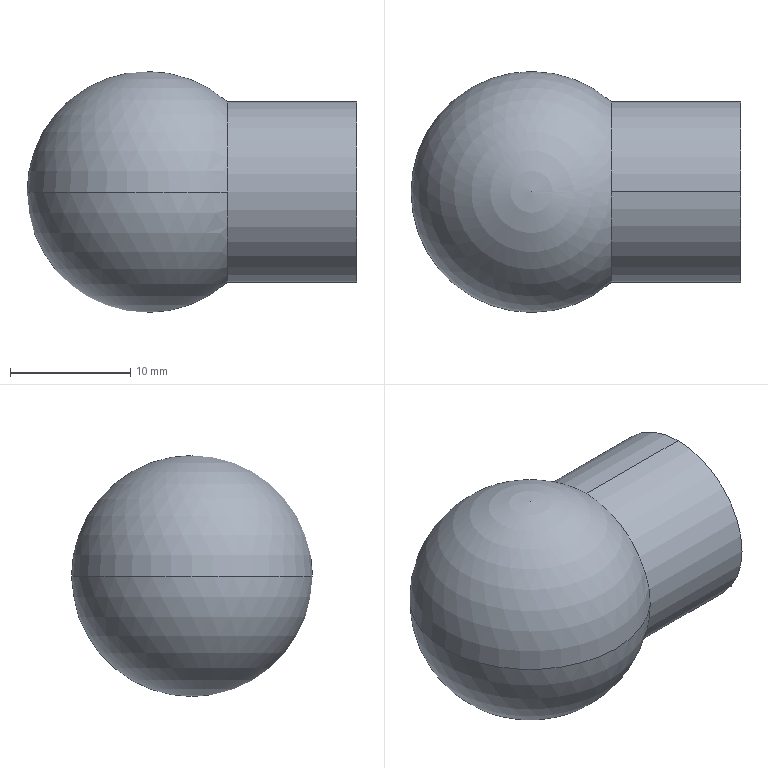Part | SolidWorks | features Revolution 2 | 1 solid | 6 faces | box 27.386 x 20 x 20 mm | volume 5453 mm3 | sphere 4 | cylinder 2 | commonest cylinder face diameters 15 x2
STEP:
#1=CARTESIAN_POINT('',(0.,-10.,0.));
#2=VERTEX_POINT('',#1);
#3=CARTESIAN_POINT('',(6.614,-7.5,0.));
#4=VERTEX_POINT('',#3);
#5=CARTESIAN_POINT('',(0.,0.,0.));
#6=DIRECTION('',(0.,0.,1.));
#7=DIRECTION('',(1.,0.,0.));
#8=AXIS2_PLACEMENT_3D('',#5,#6,#7);
#9=CIRCLE('',#8,10.);
#10=EDGE_CURVE('',#2,#4,#9,.T.);
#11=ORIENTED_EDGE('',*,*,#10,.F.);
#12=CARTESIAN_POINT('',(0.,10.,0.));
#13=VERTEX_POINT('',#12);
#14=CARTESIAN_POINT('',(0.,0.,0.));
#15=DIRECTION('',(0.,0.,-1.));
#16=DIRECTION('',(-1.,0.,0.));
#17=AXIS2_PLACEMENT_3D('',#14,#15,#16);
#18=CIRCLE('',#17,10.);
#19=EDGE_CURVE('',#2,#13,#18,.T.);
#20=ORIENTED_EDGE('',*,*,#19,.T.);
#21=CARTESIAN_POINT('',(6.614,7.5,0.));
#22=VERTEX_POINT('',#21);
#23=CARTESIAN_POINT('',(0.,0.,0.));
#24=DIRECTION('',(0.,0.,1.));
#25=DIRECTION('',(1.,0.,0.));
#26=AXIS2_PLACEMENT_3D('',#23,#24,#25);
#27=CIRCLE('',#26,10.);
#28=EDGE_CURVE('',#22,#13,#27,.T.);
#29=ORIENTED_EDGE('',*,*,#28,.F.);
#30=CARTESIAN_POINT('',(6.614,0.,-7.5));
#31=VERTEX_POINT('',#30);
#32=CARTESIAN_POINT('',(6.614,0.,0.));
#33=DIRECTION('',(1.,0.,0.));
#34=DIRECTION('',(0.,0.,-1.));
#35=AXIS2_PLACEMENT_3D('',#32,#33,#34);
#36=CIRCLE('',#35,7.5);
#37=EDGE_CURVE('',#31,#22,#36,.T.);
#38=ORIENTED_EDGE('',*,*,#37,.F.);
#39=CARTESIAN_POINT('',(6.614,0.,0.));
#40=DIRECTION('',(1.,0.,0.));
#41=DIRECTION('',(0.,0.,-1.));
#42=AXIS2_PLACEMENT_3D('',#39,#40,#41);
#43=CIRCLE('',#42,7.5);
#44=EDGE_CURVE('',#4,#31,#43,.T.);
#45=ORIENTED_EDGE('',*,*,#44,.F.);
#46=EDGE_LOOP('',(#11,#20,#29,#38,#45));
#47=FACE_OUTER_BOUND('',#46,.T.);
#48=CARTESIAN_POINT('',(0.,0.,0.));
#49=DIRECTION('',(0.,0.,-1.));
#50=DIRECTION('',(1.,0.,0.));
#51=AXIS2_PLACEMENT_3D('',#48,#49,#50);
#52=SPHERICAL_SURFACE('',#51,10.);
#53=ADVANCED_FACE('',(#47),#52,.T.);
#54=ORIENTED_EDGE('',*,*,#37,.T.);
#55=CARTESIAN_POINT('',(6.614,0.,7.5));
#56=VERTEX_POINT('',#55);
#57=CARTESIAN_POINT('',(6.614,0.,0.));
#58=DIRECTION('',(1.,0.,0.));
#59=DIRECTION('',(0.,0.,-1.));
#60=AXIS2_PLACEMENT_3D('',#57,#58,#59);
#61=CIRCLE('',#60,7.5);
#62=EDGE_CURVE('',#22,#56,#61,.T.);
#63=ORIENTED_EDGE('',*,*,#62,.T.);
#64=CARTESIAN_POINT('',(17.386,0.,7.5));
#65=VERTEX_POINT('',#64);
#66=CARTESIAN_POINT('',(27.638,0.,7.5));
#67=DIRECTION('',(1.,0.,0.));
#68=VECTOR('',#67,1000.);
#69=LINE('',#66,#68);
#70=EDGE_CURVE('',#56,#65,#69,.T.);
#71=ORIENTED_EDGE('',*,*,#70,.T.);
#72=CARTESIAN_POINT('',(17.386,7.5,0.));
#73=VERTEX_POINT('',#72);
#74=CARTESIAN_POINT('',(17.386,0.,0.));
#75=DIRECTION('',(1.,0.,0.));
#76=DIRECTION('',(0.,0.,-1.));
#77=AXIS2_PLACEMENT_3D('',#74,#75,#76);
#78=CIRCLE('',#77,7.5);
#79=EDGE_CURVE('',#73,#65,#78,.T.);
#80=ORIENTED_EDGE('',*,*,#79,.F.);
#81=CARTESIAN_POINT('',(17.386,0.,-7.5));
#82=VERTEX_POINT('',#81);
#83=CARTESIAN_POINT('',(17.386,0.,0.));
#84=DIRECTION('',(1.,0.,0.));
#85=DIRECTION('',(0.,0.,-1.));
#86=AXIS2_PLACEMENT_3D('',#83,#84,#85);
#87=CIRCLE('',#86,7.5);
#88=EDGE_CURVE('',#82,#73,#87,.T.);
#89=ORIENTED_EDGE('',*,*,#88,.F.);
#90=CARTESIAN_POINT('',(27.638,0.,-7.5));
#91=DIRECTION('',(1.,0.,0.));
#92=VECTOR('',#91,1000.);
#93=LINE('',#90,#92);
#94=EDGE_CURVE('',#31,#82,#93,.T.);
#95=ORIENTED_EDGE('',*,*,#94,.F.);
#96=EDGE_LOOP('',(#54,#63,#71,#80,#89,#95));
#97=FACE_OUTER_BOUND('',#96,.T.);
#98=CARTESIAN_POINT('',(27.638,0.,0.));
#99=DIRECTION('',(1.,0.,0.));
#100=DIRECTION('',(0.,0.,-1.));
#101=AXIS2_PLACEMENT_3D('',#98,#99,#100);
#102=CYLINDRICAL_SURFACE('',#101,7.5);
#103=ADVANCED_FACE('',(#97),#102,.T.);
#104=CARTESIAN_POINT('',(14.,0.,0.));
#105=VERTEX_POINT('',#104);
#106=CARTESIAN_POINT('',(17.386,-7.5,0.));
#107=VERTEX_POINT('',#106);
#108=CARTESIAN_POINT('',(24.,0.,0.));
#109=DIRECTION('',(0.,0.,1.));
#110=DIRECTION('',(1.,0.,0.));
#111=AXIS2_PLACEMENT_3D('',#108,#109,#110);
#112=CIRCLE('',#111,10.);
#113=EDGE_CURVE('',#105,#107,#112,.T.);
#114=ORIENTED_EDGE('',*,*,#113,.F.);
#115=CARTESIAN_POINT('',(24.,0.,0.));
#116=DIRECTION('',(0.,0.,-1.));
#117=DIRECTION('',(0.,1.,0.));
#118=AXIS2_PLACEMENT_3D('',#115,#116,#117);
#119=CIRCLE('',#118,10.);
#120=EDGE_CURVE('',#105,#73,#119,.T.);
#121=ORIENTED_EDGE('',*,*,#120,.T.);
#122=ORIENTED_EDGE('',*,*,#79,.T.);
#123=CARTESIAN_POINT('',(17.386,0.,0.));
#124=DIRECTION('',(1.,0.,0.));
#125=DIRECTION('',(0.,0.,-1.));
#126=AXIS2_PLACEMENT_3D('',#123,#124,#125);
#127=CIRCLE('',#126,7.5);
#128=EDGE_CURVE('',#65,#107,#127,.T.);
#129=ORIENTED_EDGE('',*,*,#128,.T.);
#130=EDGE_LOOP('',(#114,#121,#122,#129));
#131=FACE_OUTER_BOUND('',#130,.T.);
#132=CARTESIAN_POINT('',(24.,0.,0.));
#133=DIRECTION('',(0.,0.,-1.));
#134=DIRECTION('',(0.,-1.,0.));
#135=AXIS2_PLACEMENT_3D('',#132,#133,#134);
#136=SPHERICAL_SURFACE('',#135,10.);
#137=ADVANCED_FACE('',(#131),#136,.F.);
#138=ORIENTED_EDGE('',*,*,#120,.F.);
#139=ORIENTED_EDGE('',*,*,#113,.T.);
#140=CARTESIAN_POINT('',(17.386,0.,0.));
#141=DIRECTION('',(1.,0.,0.));
#142=DIRECTION('',(0.,0.,-1.));
#143=AXIS2_PLACEMENT_3D('',#140,#141,#142);
#144=CIRCLE('',#143,7.5);
#145=EDGE_CURVE('',#107,#82,#144,.T.);
#146=ORIENTED_EDGE('',*,*,#145,.T.);
#147=ORIENTED_EDGE('',*,*,#88,.T.);
#148=EDGE_LOOP('',(#138,#139,#146,#147));
#149=FACE_OUTER_BOUND('',#148,.T.);
#150=CARTESIAN_POINT('',(24.,0.,0.));
#151=DIRECTION('',(0.,0.,-1.));
#152=DIRECTION('',(0.,-1.,0.));
#153=AXIS2_PLACEMENT_3D('',#150,#151,#152);
#154=SPHERICAL_SURFACE('',#153,10.);
#155=ADVANCED_FACE('',(#149),#154,.F.);
#156=ORIENTED_EDGE('',*,*,#70,.F.);
#157=CARTESIAN_POINT('',(6.614,0.,0.));
#158=DIRECTION('',(1.,0.,0.));
#159=DIRECTION('',(0.,0.,-1.));
#160=AXIS2_PLACEMENT_3D('',#157,#158,#159);
#161=CIRCLE('',#160,7.5);
#162=EDGE_CURVE('',#56,#4,#161,.T.);
#163=ORIENTED_EDGE('',*,*,#162,.T.);
#164=ORIENTED_EDGE('',*,*,#44,.T.);
#165=ORIENTED_EDGE('',*,*,#94,.T.);
#166=ORIENTED_EDGE('',*,*,#145,.F.);
#167=ORIENTED_EDGE('',*,*,#128,.F.);
#168=EDGE_LOOP('',(#156,#163,#164,#165,#166,#167));
#169=FACE_OUTER_BOUND('',#168,.T.);
#170=CARTESIAN_POINT('',(27.638,0.,0.));
#171=DIRECTION('',(1.,0.,0.));
#172=DIRECTION('',(0.,0.,-1.));
#173=AXIS2_PLACEMENT_3D('',#170,#171,#172);
#174=CYLINDRICAL_SURFACE('',#173,7.5);
#175=ADVANCED_FACE('',(#169),#174,.T.);
#176=ORIENTED_EDGE('',*,*,#19,.F.);
#177=ORIENTED_EDGE('',*,*,#10,.T.);
#178=ORIENTED_EDGE('',*,*,#162,.F.);
#179=ORIENTED_EDGE('',*,*,#62,.F.);
#180=ORIENTED_EDGE('',*,*,#28,.T.);
#181=EDGE_LOOP('',(#176,#177,#178,#179,#180));
#182=FACE_OUTER_BOUND('',#181,.T.);
#183=CARTESIAN_POINT('',(0.,0.,0.));
#184=DIRECTION('',(0.,0.,-1.));
#185=DIRECTION('',(1.,0.,0.));
#186=AXIS2_PLACEMENT_3D('',#183,#184,#185);
#187=SPHERICAL_SURFACE('',#186,10.);
#188=ADVANCED_FACE('',(#182),#187,.T.);
#189=CLOSED_SHELL('',(#53,#103,#137,#155,#175,#188));
#190=MANIFOLD_SOLID_BREP('',#189);
#191=CARTESIAN_POINT('',(0.,0.,0.));
#192=DIRECTION('',(0.,0.,1.));
#193=DIRECTION('',(1.,0.,0.));
#194=AXIS2_PLACEMENT_3D('',#191,#192,#193);
#195=(LENGTH_UNIT()NAMED_UNIT(*)SI_UNIT(.MILLI.,.METRE.));
#196=UNCERTAINTY_MEASURE_WITH_UNIT(LENGTH_MEASURE(0.00001),#195,'','');
#197=(NAMED_UNIT(*)PLANE_ANGLE_UNIT()SI_UNIT($,.RADIAN.));
#198=(NAMED_UNIT(*)SI_UNIT($,.STERADIAN.)SOLID_ANGLE_UNIT());
#199=(GEOMETRIC_REPRESENTATION_CONTEXT(3)GLOBAL_UNCERTAINTY_ASSIGNED_CONTEXT((#196))GLOBAL_UNIT_ASSIGNED_CONTEXT((#195,#197,#198))REPRESENTATION_CONTEXT('',''));
#200=ADVANCED_BREP_SHAPE_REPRESENTATION('',(#190,#194),#199);